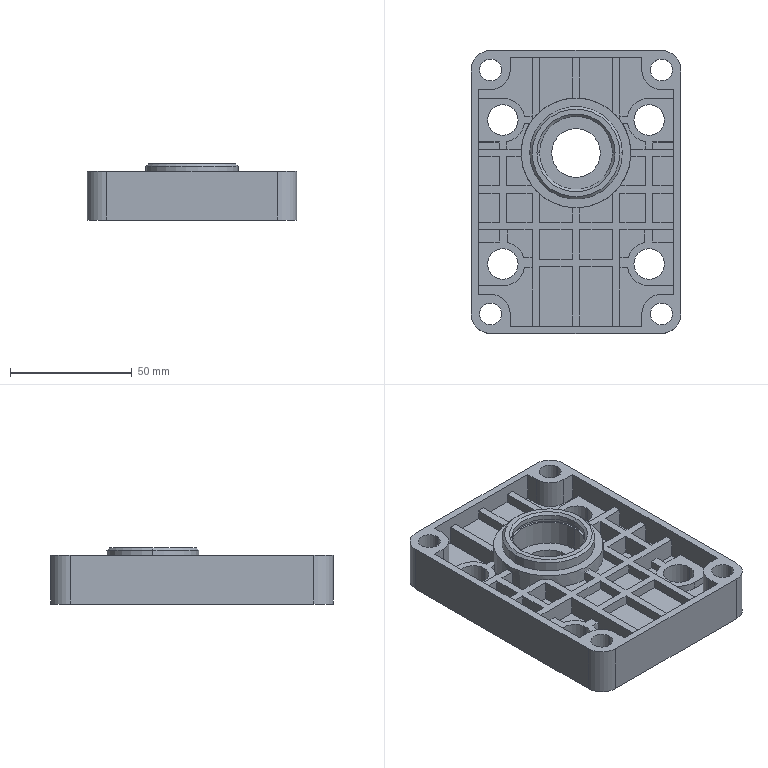Part | SolidWorks | features ICE 9, MirrorPattern 2, Chamfer 1, Extrusion 1, RevCut 1 | 1 solid | 195 faces | box 86 x 116 x 23 mm | volume 118984 mm3 | plane 143 | cylinder 48 | cone 4 | commonest cylinder face diameters 9 x8 12.5 x8 16 x8 18 x8 8 x4 30 x4